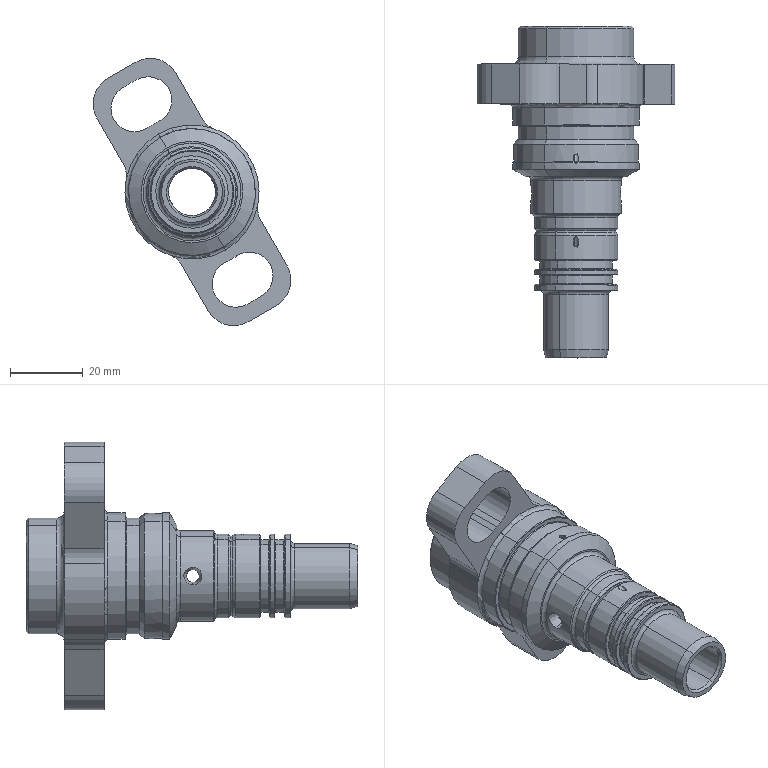Part | SolidWorks | features BaseBody 1 | 1 solid | 169 faces | box 54.543 x 91.5 x 73.761 mm | volume 42133 mm3 | cylinder 72 | cone 39 | torus 35 | plane 23 | commonest cylinder face diameters 13 x10 1.5 x8 23 x8 3.5 x4 12 x4 16 x4